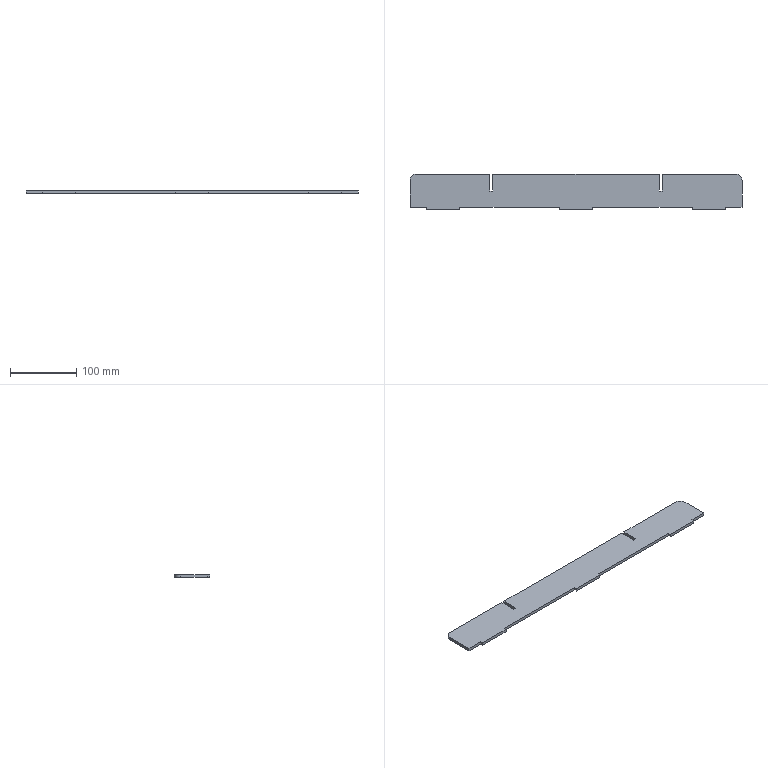Part | SolidWorks | features FlatPattern 1, SMBaseFlange 1, SheetMetal 1 | 1 solid | 28 faces | box 500 x 54 x 4.5 mm | volume 113974 mm3 | plane 26 | cylinder 2 | commonest cylinder face diameters 20 x2
STEP:
#1=CARTESIAN_POINT('',(-710.,249.731,0.));
#2=VERTEX_POINT('',#1);
#3=CARTESIAN_POINT('',(-685.,249.731,0.));
#4=VERTEX_POINT('',#3);
#5=CARTESIAN_POINT('',(-685.,249.731,0.));
#6=DIRECTION('',(1.,0.,0.));
#7=VECTOR('',#6,1000.);
#8=LINE('',#5,#7);
#9=EDGE_CURVE('',#2,#4,#8,.T.);
#10=ORIENTED_EDGE('',*,*,#9,.F.);
#11=CARTESIAN_POINT('',(-710.,249.731,-4.5));
#12=VERTEX_POINT('',#11);
#13=CARTESIAN_POINT('',(-710.,249.731,-4.5));
#14=DIRECTION('',(0.,0.,1.));
#15=VECTOR('',#14,1000.);
#16=LINE('',#13,#15);
#17=EDGE_CURVE('',#12,#2,#16,.T.);
#18=ORIENTED_EDGE('',*,*,#17,.F.);
#19=CARTESIAN_POINT('',(-685.,249.731,-4.5));
#20=VERTEX_POINT('',#19);
#21=CARTESIAN_POINT('',(-685.,249.731,-4.5));
#22=DIRECTION('',(1.,0.,0.));
#23=VECTOR('',#22,1000.);
#24=LINE('',#21,#23);
#25=EDGE_CURVE('',#12,#20,#24,.T.);
#26=ORIENTED_EDGE('',*,*,#25,.T.);
#27=CARTESIAN_POINT('',(-685.,249.731,-4.5));
#28=DIRECTION('',(0.,0.,1.));
#29=VECTOR('',#28,1000.);
#30=LINE('',#27,#29);
#31=EDGE_CURVE('',#20,#4,#30,.T.);
#32=ORIENTED_EDGE('',*,*,#31,.T.);
#33=EDGE_LOOP('',(#10,#18,#26,#32));
#34=FACE_OUTER_BOUND('',#33,.T.);
#35=CARTESIAN_POINT('',(-685.,249.731,-4.5));
#36=DIRECTION('',(0.,-1.,0.));
#37=DIRECTION('',(0.,0.,-1.));
#38=AXIS2_PLACEMENT_3D('',#35,#36,#37);
#39=PLANE('',#38);
#40=ADVANCED_FACE('',(#34),#39,.T.);
#41=CARTESIAN_POINT('',(-710.,289.731,0.));
#42=VERTEX_POINT('',#41);
#43=CARTESIAN_POINT('',(-710.,249.731,0.));
#44=DIRECTION('',(0.,-1.,0.));
#45=VECTOR('',#44,1000.);
#46=LINE('',#43,#45);
#47=EDGE_CURVE('',#42,#2,#46,.T.);
#48=ORIENTED_EDGE('',*,*,#47,.F.);
#49=CARTESIAN_POINT('',(-710.,289.731,-4.5));
#50=VERTEX_POINT('',#49);
#51=CARTESIAN_POINT('',(-710.,289.731,-4.5));
#52=DIRECTION('',(0.,0.,1.));
#53=VECTOR('',#52,1000.);
#54=LINE('',#51,#53);
#55=EDGE_CURVE('',#50,#42,#54,.T.);
#56=ORIENTED_EDGE('',*,*,#55,.F.);
#57=CARTESIAN_POINT('',(-710.,249.731,-4.5));
#58=DIRECTION('',(0.,-1.,0.));
#59=VECTOR('',#58,1000.);
#60=LINE('',#57,#59);
#61=EDGE_CURVE('',#50,#12,#60,.T.);
#62=ORIENTED_EDGE('',*,*,#61,.T.);
#63=ORIENTED_EDGE('',*,*,#17,.T.);
#64=EDGE_LOOP('',(#48,#56,#62,#63));
#65=FACE_OUTER_BOUND('',#64,.T.);
#66=CARTESIAN_POINT('',(-710.,249.731,-4.5));
#67=DIRECTION('',(-1.,0.,0.));
#68=DIRECTION('',(0.,0.,1.));
#69=AXIS2_PLACEMENT_3D('',#66,#67,#68);
#70=PLANE('',#69);
#71=ADVANCED_FACE('',(#65),#70,.T.);
#72=CARTESIAN_POINT('',(-700.,299.731,0.));
#73=VERTEX_POINT('',#72);
#74=CARTESIAN_POINT('',(-700.,289.731,0.));
#75=DIRECTION('',(0.,0.,1.));
#76=DIRECTION('',(-1.,0.,0.));
#77=AXIS2_PLACEMENT_3D('',#74,#75,#76);
#78=CIRCLE('',#77,10.);
#79=EDGE_CURVE('',#73,#42,#78,.T.);
#80=ORIENTED_EDGE('',*,*,#79,.F.);
#81=CARTESIAN_POINT('',(-700.,299.731,-4.5));
#82=VERTEX_POINT('',#81);
#83=CARTESIAN_POINT('',(-700.,299.731,-4.5));
#84=DIRECTION('',(0.,0.,1.));
#85=VECTOR('',#84,1000.);
#86=LINE('',#83,#85);
#87=EDGE_CURVE('',#82,#73,#86,.T.);
#88=ORIENTED_EDGE('',*,*,#87,.F.);
#89=CARTESIAN_POINT('',(-700.,289.731,-4.5));
#90=DIRECTION('',(0.,0.,1.));
#91=DIRECTION('',(-1.,0.,0.));
#92=AXIS2_PLACEMENT_3D('',#89,#90,#91);
#93=CIRCLE('',#92,10.);
#94=EDGE_CURVE('',#82,#50,#93,.T.);
#95=ORIENTED_EDGE('',*,*,#94,.T.);
#96=ORIENTED_EDGE('',*,*,#55,.T.);
#97=EDGE_LOOP('',(#80,#88,#95,#96));
#98=FACE_OUTER_BOUND('',#97,.T.);
#99=CARTESIAN_POINT('',(-700.,289.731,-4.5));
#100=DIRECTION('',(0.,0.,1.));
#101=DIRECTION('',(1.,0.,0.));
#102=AXIS2_PLACEMENT_3D('',#99,#100,#101);
#103=CYLINDRICAL_SURFACE('',#102,10.);
#104=ADVANCED_FACE('',(#98),#103,.T.);
#105=CARTESIAN_POINT('',(-590.,299.731,0.));
#106=VERTEX_POINT('',#105);
#107=CARTESIAN_POINT('',(-700.,299.731,0.));
#108=DIRECTION('',(-1.,0.,0.));
#109=VECTOR('',#108,1000.);
#110=LINE('',#107,#109);
#111=EDGE_CURVE('',#106,#73,#110,.T.);
#112=ORIENTED_EDGE('',*,*,#111,.F.);
#113=CARTESIAN_POINT('',(-590.,299.731,-4.5));
#114=VERTEX_POINT('',#113);
#115=CARTESIAN_POINT('',(-590.,299.731,-4.5));
#116=DIRECTION('',(0.,0.,1.));
#117=VECTOR('',#116,1000.);
#118=LINE('',#115,#117);
#119=EDGE_CURVE('',#114,#106,#118,.T.);
#120=ORIENTED_EDGE('',*,*,#119,.F.);
#121=CARTESIAN_POINT('',(-700.,299.731,-4.5));
#122=DIRECTION('',(-1.,0.,0.));
#123=VECTOR('',#122,1000.);
#124=LINE('',#121,#123);
#125=EDGE_CURVE('',#114,#82,#124,.T.);
#126=ORIENTED_EDGE('',*,*,#125,.T.);
#127=ORIENTED_EDGE('',*,*,#87,.T.);
#128=EDGE_LOOP('',(#112,#120,#126,#127));
#129=FACE_OUTER_BOUND('',#128,.T.);
#130=CARTESIAN_POINT('',(-700.,299.731,-4.5));
#131=DIRECTION('',(0.,1.,0.));
#132=DIRECTION('',(-1.,0.,0.));
#133=AXIS2_PLACEMENT_3D('',#130,#131,#132);
#134=PLANE('',#133);
#135=ADVANCED_FACE('',(#129),#134,.T.);
#136=CARTESIAN_POINT('',(-590.,274.231,0.));
#137=VERTEX_POINT('',#136);
#138=CARTESIAN_POINT('',(-590.,299.731,0.));
#139=DIRECTION('',(0.,1.,0.));
#140=VECTOR('',#139,1000.);
#141=LINE('',#138,#140);
#142=EDGE_CURVE('',#137,#106,#141,.T.);
#143=ORIENTED_EDGE('',*,*,#142,.F.);
#144=CARTESIAN_POINT('',(-590.,274.231,-4.5));
#145=VERTEX_POINT('',#144);
#146=CARTESIAN_POINT('',(-590.,274.231,-4.5));
#147=DIRECTION('',(0.,0.,1.));
#148=VECTOR('',#147,1000.);
#149=LINE('',#146,#148);
#150=EDGE_CURVE('',#145,#137,#149,.T.);
#151=ORIENTED_EDGE('',*,*,#150,.F.);
#152=CARTESIAN_POINT('',(-590.,299.731,-4.5));
#153=DIRECTION('',(0.,1.,0.));
#154=VECTOR('',#153,1000.);
#155=LINE('',#152,#154);
#156=EDGE_CURVE('',#145,#114,#155,.T.);
#157=ORIENTED_EDGE('',*,*,#156,.T.);
#158=ORIENTED_EDGE('',*,*,#119,.T.);
#159=EDGE_LOOP('',(#143,#151,#157,#158));
#160=FACE_OUTER_BOUND('',#159,.T.);
#161=CARTESIAN_POINT('',(-590.,299.731,-4.5));
#162=DIRECTION('',(1.,0.,0.));
#163=DIRECTION('',(0.,0.,-1.));
#164=AXIS2_PLACEMENT_3D('',#161,#162,#163);
#165=PLANE('',#164);
#166=ADVANCED_FACE('',(#160),#165,.T.);
#167=CARTESIAN_POINT('',(-585.5,274.231,0.));
#168=VERTEX_POINT('',#167);
#169=CARTESIAN_POINT('',(-590.,274.231,0.));
#170=DIRECTION('',(-1.,0.,0.));
#171=VECTOR('',#170,1000.);
#172=LINE('',#169,#171);
#173=EDGE_CURVE('',#168,#137,#172,.T.);
#174=ORIENTED_EDGE('',*,*,#173,.F.);
#175=CARTESIAN_POINT('',(-585.5,274.231,-4.5));
#176=VERTEX_POINT('',#175);
#177=CARTESIAN_POINT('',(-585.5,274.231,-4.5));
#178=DIRECTION('',(0.,0.,1.));
#179=VECTOR('',#178,1000.);
#180=LINE('',#177,#179);
#181=EDGE_CURVE('',#176,#168,#180,.T.);
#182=ORIENTED_EDGE('',*,*,#181,.F.);
#183=CARTESIAN_POINT('',(-590.,274.231,-4.5));
#184=DIRECTION('',(-1.,0.,0.));
#185=VECTOR('',#184,1000.);
#186=LINE('',#183,#185);
#187=EDGE_CURVE('',#176,#145,#186,.T.);
#188=ORIENTED_EDGE('',*,*,#187,.T.);
#189=ORIENTED_EDGE('',*,*,#150,.T.);
#190=EDGE_LOOP('',(#174,#182,#188,#189));
#191=FACE_OUTER_BOUND('',#190,.T.);
#192=CARTESIAN_POINT('',(-590.,274.231,-4.5));
#193=DIRECTION('',(0.,1.,0.));
#194=DIRECTION('',(0.,0.,1.));
#195=AXIS2_PLACEMENT_3D('',#192,#193,#194);
#196=PLANE('',#195);
#197=ADVANCED_FACE('',(#191),#196,.T.);
#198=CARTESIAN_POINT('',(-585.5,299.731,0.));
#199=VERTEX_POINT('',#198);
#200=CARTESIAN_POINT('',(-585.5,274.231,0.));
#201=DIRECTION('',(0.,-1.,0.));
#202=VECTOR('',#201,1000.);
#203=LINE('',#200,#202);
#204=EDGE_CURVE('',#199,#168,#203,.T.);
#205=ORIENTED_EDGE('',*,*,#204,.F.);
#206=CARTESIAN_POINT('',(-585.5,299.731,-4.5));
#207=VERTEX_POINT('',#206);
#208=CARTESIAN_POINT('',(-585.5,299.731,-4.5));
#209=DIRECTION('',(0.,0.,1.));
#210=VECTOR('',#209,1000.);
#211=LINE('',#208,#210);
#212=EDGE_CURVE('',#207,#199,#211,.T.);
#213=ORIENTED_EDGE('',*,*,#212,.F.);
#214=CARTESIAN_POINT('',(-585.5,274.231,-4.5));
#215=DIRECTION('',(0.,-1.,0.));
#216=VECTOR('',#215,1000.);
#217=LINE('',#214,#216);
#218=EDGE_CURVE('',#207,#176,#217,.T.);
#219=ORIENTED_EDGE('',*,*,#218,.T.);
#220=ORIENTED_EDGE('',*,*,#181,.T.);
#221=EDGE_LOOP('',(#205,#213,#219,#220));
#222=FACE_OUTER_BOUND('',#221,.T.);
#223=CARTESIAN_POINT('',(-585.5,274.231,-4.5));
#224=DIRECTION('',(-1.,0.,0.));
#225=DIRECTION('',(0.,0.,1.));
#226=AXIS2_PLACEMENT_3D('',#223,#224,#225);
#227=PLANE('',#226);
#228=ADVANCED_FACE('',(#222),#227,.T.);
#229=CARTESIAN_POINT('',(-334.5,299.731,0.));
#230=VERTEX_POINT('',#229);
#231=CARTESIAN_POINT('',(-585.5,299.731,0.));
#232=DIRECTION('',(-1.,0.,0.));
#233=VECTOR('',#232,1000.);
#234=LINE('',#231,#233);
#235=EDGE_CURVE('',#230,#199,#234,.T.);
#236=ORIENTED_EDGE('',*,*,#235,.F.);
#237=CARTESIAN_POINT('',(-334.5,299.731,-4.5));
#238=VERTEX_POINT('',#237);
#239=CARTESIAN_POINT('',(-334.5,299.731,-4.5));
#240=DIRECTION('',(0.,0.,1.));
#241=VECTOR('',#240,1000.);
#242=LINE('',#239,#241);
#243=EDGE_CURVE('',#238,#230,#242,.T.);
#244=ORIENTED_EDGE('',*,*,#243,.F.);
#245=CARTESIAN_POINT('',(-585.5,299.731,-4.5));
#246=DIRECTION('',(-1.,0.,0.));
#247=VECTOR('',#246,1000.);
#248=LINE('',#245,#247);
#249=EDGE_CURVE('',#238,#207,#248,.T.);
#250=ORIENTED_EDGE('',*,*,#249,.T.);
#251=ORIENTED_EDGE('',*,*,#212,.T.);
#252=EDGE_LOOP('',(#236,#244,#250,#251));
#253=FACE_OUTER_BOUND('',#252,.T.);
#254=CARTESIAN_POINT('',(-585.5,299.731,-4.5));
#255=DIRECTION('',(0.,1.,0.));
#256=DIRECTION('',(-1.,0.,0.));
#257=AXIS2_PLACEMENT_3D('',#254,#255,#256);
#258=PLANE('',#257);
#259=ADVANCED_FACE('',(#253),#258,.T.);
#260=CARTESIAN_POINT('',(-334.5,274.231,0.));
#261=VERTEX_POINT('',#260);
#262=CARTESIAN_POINT('',(-334.5,299.731,0.));
#263=DIRECTION('',(0.,1.,0.));
#264=VECTOR('',#263,1000.);
#265=LINE('',#262,#264);
#266=EDGE_CURVE('',#261,#230,#265,.T.);
#267=ORIENTED_EDGE('',*,*,#266,.F.);
#268=CARTESIAN_POINT('',(-334.5,274.231,-4.5));
#269=VERTEX_POINT('',#268);
#270=CARTESIAN_POINT('',(-334.5,274.231,-4.5));
#271=DIRECTION('',(0.,0.,1.));
#272=VECTOR('',#271,1000.);
#273=LINE('',#270,#272);
#274=EDGE_CURVE('',#269,#261,#273,.T.);
#275=ORIENTED_EDGE('',*,*,#274,.F.);
#276=CARTESIAN_POINT('',(-334.5,299.731,-4.5));
#277=DIRECTION('',(0.,1.,0.));
#278=VECTOR('',#277,1000.);
#279=LINE('',#276,#278);
#280=EDGE_CURVE('',#269,#238,#279,.T.);
#281=ORIENTED_EDGE('',*,*,#280,.T.);
#282=ORIENTED_EDGE('',*,*,#243,.T.);
#283=EDGE_LOOP('',(#267,#275,#281,#282));
#284=FACE_OUTER_BOUND('',#283,.T.);
#285=CARTESIAN_POINT('',(-334.5,299.731,-4.5));
#286=DIRECTION('',(1.,0.,0.));
#287=DIRECTION('',(0.,1.,0.));
#288=AXIS2_PLACEMENT_3D('',#285,#286,#287);
#289=PLANE('',#288);
#290=ADVANCED_FACE('',(#284),#289,.T.);
#291=CARTESIAN_POINT('',(-330.,274.231,0.));
#292=VERTEX_POINT('',#291);
#293=CARTESIAN_POINT('',(-334.5,274.231,0.));
#294=DIRECTION('',(-1.,0.,0.));
#295=VECTOR('',#294,1000.);
#296=LINE('',#293,#295);
#297=EDGE_CURVE('',#292,#261,#296,.T.);
#298=ORIENTED_EDGE('',*,*,#297,.F.);
#299=CARTESIAN_POINT('',(-330.,274.231,-4.5));
#300=VERTEX_POINT('',#299);
#301=CARTESIAN_POINT('',(-330.,274.231,-4.5));
#302=DIRECTION('',(0.,0.,1.));
#303=VECTOR('',#302,1000.);
#304=LINE('',#301,#303);
#305=EDGE_CURVE('',#300,#292,#304,.T.);
#306=ORIENTED_EDGE('',*,*,#305,.F.);
#307=CARTESIAN_POINT('',(-334.5,274.231,-4.5));
#308=DIRECTION('',(-1.,0.,0.));
#309=VECTOR('',#308,1000.);
#310=LINE('',#307,#309);
#311=EDGE_CURVE('',#300,#269,#310,.T.);
#312=ORIENTED_EDGE('',*,*,#311,.T.);
#313=ORIENTED_EDGE('',*,*,#274,.T.);
#314=EDGE_LOOP('',(#298,#306,#312,#313));
#315=FACE_OUTER_BOUND('',#314,.T.);
#316=CARTESIAN_POINT('',(-334.5,274.231,-4.5));
#317=DIRECTION('',(0.,1.,0.));
#318=DIRECTION('',(0.,0.,1.));
#319=AXIS2_PLACEMENT_3D('',#316,#317,#318);
#320=PLANE('',#319);
#321=ADVANCED_FACE('',(#315),#320,.T.);
#322=CARTESIAN_POINT('',(-330.,299.731,0.));
#323=VERTEX_POINT('',#322);
#324=CARTESIAN_POINT('',(-330.,274.231,0.));
#325=DIRECTION('',(0.,-1.,0.));
#326=VECTOR('',#325,1000.);
#327=LINE('',#324,#326);
#328=EDGE_CURVE('',#323,#292,#327,.T.);
#329=ORIENTED_EDGE('',*,*,#328,.F.);
#330=CARTESIAN_POINT('',(-330.,299.731,-4.5));
#331=VERTEX_POINT('',#330);
#332=CARTESIAN_POINT('',(-330.,299.731,-4.5));
#333=DIRECTION('',(0.,0.,1.));
#334=VECTOR('',#333,1000.);
#335=LINE('',#332,#334);
#336=EDGE_CURVE('',#331,#323,#335,.T.);
#337=ORIENTED_EDGE('',*,*,#336,.F.);
#338=CARTESIAN_POINT('',(-330.,274.231,-4.5));
#339=DIRECTION('',(0.,-1.,0.));
#340=VECTOR('',#339,1000.);
#341=LINE('',#338,#340);
#342=EDGE_CURVE('',#331,#300,#341,.T.);
#343=ORIENTED_EDGE('',*,*,#342,.T.);
#344=ORIENTED_EDGE('',*,*,#305,.T.);
#345=EDGE_LOOP('',(#329,#337,#343,#344));
#346=FACE_OUTER_BOUND('',#345,.T.);
#347=CARTESIAN_POINT('',(-330.,274.231,-4.5));
#348=DIRECTION('',(-1.,0.,0.));
#349=DIRECTION('',(0.,-1.,0.));
#350=AXIS2_PLACEMENT_3D('',#347,#348,#349);
#351=PLANE('',#350);
#352=ADVANCED_FACE('',(#346),#351,.T.);
#353=CARTESIAN_POINT('',(-220.,299.731,0.));
#354=VERTEX_POINT('',#353);
#355=CARTESIAN_POINT('',(-330.,299.731,0.));
#356=DIRECTION('',(-1.,0.,0.));
#357=VECTOR('',#356,1000.);
#358=LINE('',#355,#357);
#359=EDGE_CURVE('',#354,#323,#358,.T.);
#360=ORIENTED_EDGE('',*,*,#359,.F.);
#361=CARTESIAN_POINT('',(-220.,299.731,-4.5));
#362=VERTEX_POINT('',#361);
#363=CARTESIAN_POINT('',(-220.,299.731,-4.5));
#364=DIRECTION('',(0.,0.,1.));
#365=VECTOR('',#364,1000.);
#366=LINE('',#363,#365);
#367=EDGE_CURVE('',#362,#354,#366,.T.);
#368=ORIENTED_EDGE('',*,*,#367,.F.);
#369=CARTESIAN_POINT('',(-330.,299.731,-4.5));
#370=DIRECTION('',(-1.,0.,0.));
#371=VECTOR('',#370,1000.);
#372=LINE('',#369,#371);
#373=EDGE_CURVE('',#362,#331,#372,.T.);
#374=ORIENTED_EDGE('',*,*,#373,.T.);
#375=ORIENTED_EDGE('',*,*,#336,.T.);
#376=EDGE_LOOP('',(#360,#368,#374,#375));
#377=FACE_OUTER_BOUND('',#376,.T.);
#378=CARTESIAN_POINT('',(-330.,299.731,-4.5));
#379=DIRECTION('',(0.,1.,0.));
#380=DIRECTION('',(-1.,0.,0.));
#381=AXIS2_PLACEMENT_3D('',#378,#379,#380);
#382=PLANE('',#381);
#383=ADVANCED_FACE('',(#377),#382,.T.);
#384=CARTESIAN_POINT('',(-210.,289.731,0.));
#385=VERTEX_POINT('',#384);
#386=CARTESIAN_POINT('',(-220.,289.731,0.));
#387=DIRECTION('',(0.,0.,1.));
#388=DIRECTION('',(-1.,0.,0.));
#389=AXIS2_PLACEMENT_3D('',#386,#387,#388);
#390=CIRCLE('',#389,10.);
#391=EDGE_CURVE('',#385,#354,#390,.T.);
#392=ORIENTED_EDGE('',*,*,#391,.F.);
#393=CARTESIAN_POINT('',(-210.,289.731,-4.5));
#394=VERTEX_POINT('',#393);
#395=CARTESIAN_POINT('',(-210.,289.731,-4.5));
#396=DIRECTION('',(0.,0.,1.));
#397=VECTOR('',#396,1000.);
#398=LINE('',#395,#397);
#399=EDGE_CURVE('',#394,#385,#398,.T.);
#400=ORIENTED_EDGE('',*,*,#399,.F.);
#401=CARTESIAN_POINT('',(-220.,289.731,-4.5));
#402=DIRECTION('',(0.,0.,1.));
#403=DIRECTION('',(-1.,0.,0.));
#404=AXIS2_PLACEMENT_3D('',#401,#402,#403);
#405=CIRCLE('',#404,10.);
#406=EDGE_CURVE('',#394,#362,#405,.T.);
#407=ORIENTED_EDGE('',*,*,#406,.T.);
#408=ORIENTED_EDGE('',*,*,#367,.T.);
#409=EDGE_LOOP('',(#392,#400,#407,#408));
#410=FACE_OUTER_BOUND('',#409,.T.);
#411=CARTESIAN_POINT('',(-220.,289.731,-4.5));
#412=DIRECTION('',(0.,0.,1.));
#413=DIRECTION('',(1.,0.,0.));
#414=AXIS2_PLACEMENT_3D('',#411,#412,#413);
#415=CYLINDRICAL_SURFACE('',#414,10.);
#416=ADVANCED_FACE('',(#410),#415,.T.);
#417=CARTESIAN_POINT('',(-210.,249.731,0.));
#418=VERTEX_POINT('',#417);
#419=CARTESIAN_POINT('',(-210.,289.731,0.));
#420=DIRECTION('',(0.,1.,0.));
#421=VECTOR('',#420,1000.);
#422=LINE('',#419,#421);
#423=EDGE_CURVE('',#418,#385,#422,.T.);
#424=ORIENTED_EDGE('',*,*,#423,.F.);
#425=CARTESIAN_POINT('',(-210.,249.731,-4.5));
#426=VERTEX_POINT('',#425);
#427=CARTESIAN_POINT('',(-210.,249.731,-4.5));
#428=DIRECTION('',(0.,0.,1.));
#429=VECTOR('',#428,1000.);
#430=LINE('',#427,#429);
#431=EDGE_CURVE('',#426,#418,#430,.T.);
#432=ORIENTED_EDGE('',*,*,#431,.F.);
#433=CARTESIAN_POINT('',(-210.,289.731,-4.5));
#434=DIRECTION('',(0.,1.,0.));
#435=VECTOR('',#434,1000.);
#436=LINE('',#433,#435);
#437=EDGE_CURVE('',#426,#394,#436,.T.);
#438=ORIENTED_EDGE('',*,*,#437,.T.);
#439=ORIENTED_EDGE('',*,*,#399,.T.);
#440=EDGE_LOOP('',(#424,#432,#438,#439));
#441=FACE_OUTER_BOUND('',#440,.T.);
#442=CARTESIAN_POINT('',(-210.,289.731,-4.5));
#443=DIRECTION('',(1.,0.,0.));
#444=DIRECTION('',(0.,1.,0.));
#445=AXIS2_PLACEMENT_3D('',#442,#443,#444);
#446=PLANE('',#445);
#447=ADVANCED_FACE('',(#441),#446,.T.);
#448=CARTESIAN_POINT('',(-235.,249.731,0.));
#449=VERTEX_POINT('',#448);
#450=CARTESIAN_POINT('',(-210.,249.731,0.));
#451=DIRECTION('',(1.,0.,0.));
#452=VECTOR('',#451,1000.);
#453=LINE('',#450,#452);
#454=EDGE_CURVE('',#449,#418,#453,.T.);
#455=ORIENTED_EDGE('',*,*,#454,.F.);
#456=CARTESIAN_POINT('',(-235.,249.731,-4.5));
#457=VERTEX_POINT('',#456);
#458=CARTESIAN_POINT('',(-235.,249.731,-4.5));
#459=DIRECTION('',(0.,0.,1.));
#460=VECTOR('',#459,1000.);
#461=LINE('',#458,#460);
#462=EDGE_CURVE('',#457,#449,#461,.T.);
#463=ORIENTED_EDGE('',*,*,#462,.F.);
#464=CARTESIAN_POINT('',(-210.,249.731,-4.5));
#465=DIRECTION('',(1.,0.,0.));
#466=VECTOR('',#465,1000.);
#467=LINE('',#464,#466);
#468=EDGE_CURVE('',#457,#426,#467,.T.);
#469=ORIENTED_EDGE('',*,*,#468,.T.);
#470=ORIENTED_EDGE('',*,*,#431,.T.);
#471=EDGE_LOOP('',(#455,#463,#469,#470));
#472=FACE_OUTER_BOUND('',#471,.T.);
#473=CARTESIAN_POINT('',(-210.,249.731,-4.5));
#474=DIRECTION('',(0.,-1.,0.));
#475=DIRECTION('',(1.,0.,0.));
#476=AXIS2_PLACEMENT_3D('',#473,#474,#475);
#477=PLANE('',#476);
#478=ADVANCED_FACE('',(#472),#477,.T.);
#479=CARTESIAN_POINT('',(-235.,245.731,0.));
#480=VERTEX_POINT('',#479);
#481=CARTESIAN_POINT('',(-235.,245.731,0.));
#482=DIRECTION('',(0.,1.,0.));
#483=VECTOR('',#482,1000.);
#484=LINE('',#481,#483);
#485=EDGE_CURVE('',#480,#449,#484,.T.);
#486=ORIENTED_EDGE('',*,*,#485,.F.);
#487=CARTESIAN_POINT('',(-235.,245.731,-4.5));
#488=VERTEX_POINT('',#487);
#489=CARTESIAN_POINT('',(-235.,245.731,-4.5));
#490=DIRECTION('',(0.,0.,1.));
#491=VECTOR('',#490,1000.);
#492=LINE('',#489,#491);
#493=EDGE_CURVE('',#488,#480,#492,.T.);
#494=ORIENTED_EDGE('',*,*,#493,.F.);
#495=CARTESIAN_POINT('',(-235.,245.731,-4.5));
#496=DIRECTION('',(0.,1.,0.));
#497=VECTOR('',#496,1000.);
#498=LINE('',#495,#497);
#499=EDGE_CURVE('',#488,#457,#498,.T.);
#500=ORIENTED_EDGE('',*,*,#499,.T.);
#501=ORIENTED_EDGE('',*,*,#462,.T.);
#502=EDGE_LOOP('',(#486,#494,#500,#501));
#503=FACE_OUTER_BOUND('',#502,.T.);
#504=CARTESIAN_POINT('',(-235.,245.731,-4.5));
#505=DIRECTION('',(1.,0.,0.));
#506=DIRECTION('',(0.,0.,-1.));
#507=AXIS2_PLACEMENT_3D('',#504,#505,#506);
#508=PLANE('',#507);
#509=ADVANCED_FACE('',(#503),#508,.T.);
#510=CARTESIAN_POINT('',(-285.,245.731,0.));
#511=VERTEX_POINT('',#510);
#512=CARTESIAN_POINT('',(-285.,245.731,0.));
#513=DIRECTION('',(1.,0.,0.));
#514=VECTOR('',#513,1000.);
#515=LINE('',#512,#514);
#516=EDGE_CURVE('',#511,#480,#515,.T.);
#517=ORIENTED_EDGE('',*,*,#516,.F.);
#518=CARTESIAN_POINT('',(-285.,245.731,-4.5));
#519=VERTEX_POINT('',#518);
#520=CARTESIAN_POINT('',(-285.,245.731,-4.5));
#521=DIRECTION('',(0.,0.,1.));
#522=VECTOR('',#521,1000.);
#523=LINE('',#520,#522);
#524=EDGE_CURVE('',#519,#511,#523,.T.);
#525=ORIENTED_EDGE('',*,*,#524,.F.);
#526=CARTESIAN_POINT('',(-285.,245.731,-4.5));
#527=DIRECTION('',(1.,0.,0.));
#528=VECTOR('',#527,1000.);
#529=LINE('',#526,#528);
#530=EDGE_CURVE('',#519,#488,#529,.T.);
#531=ORIENTED_EDGE('',*,*,#530,.T.);
#532=ORIENTED_EDGE('',*,*,#493,.T.);
#533=EDGE_LOOP('',(#517,#525,#531,#532));
#534=FACE_OUTER_BOUND('',#533,.T.);
#535=CARTESIAN_POINT('',(-285.,245.731,-4.5));
#536=DIRECTION('',(0.,-1.,0.));
#537=DIRECTION('',(0.,0.,-1.));
#538=AXIS2_PLACEMENT_3D('',#535,#536,#537);
#539=PLANE('',#538);
#540=ADVANCED_FACE('',(#534),#539,.T.);
#541=CARTESIAN_POINT('',(-285.,249.731,0.));
#542=VERTEX_POINT('',#541);
#543=CARTESIAN_POINT('',(-285.,249.731,0.));
#544=DIRECTION('',(0.,-1.,0.));
#545=VECTOR('',#544,1000.);
#546=LINE('',#543,#545);
#547=EDGE_CURVE('',#542,#511,#546,.T.);
#548=ORIENTED_EDGE('',*,*,#547,.F.);
#549=CARTESIAN_POINT('',(-285.,249.731,-4.5));
#550=VERTEX_POINT('',#549);
#551=CARTESIAN_POINT('',(-285.,249.731,-4.5));
#552=DIRECTION('',(0.,0.,1.));
#553=VECTOR('',#552,1000.);
#554=LINE('',#551,#553);
#555=EDGE_CURVE('',#550,#542,#554,.T.);
#556=ORIENTED_EDGE('',*,*,#555,.F.);
#557=CARTESIAN_POINT('',(-285.,249.731,-4.5));
#558=DIRECTION('',(0.,-1.,0.));
#559=VECTOR('',#558,1000.);
#560=LINE('',#557,#559);
#561=EDGE_CURVE('',#550,#519,#560,.T.);
#562=ORIENTED_EDGE('',*,*,#561,.T.);
#563=ORIENTED_EDGE('',*,*,#524,.T.);
#564=EDGE_LOOP('',(#548,#556,#562,#563));
#565=FACE_OUTER_BOUND('',#564,.T.);
#566=CARTESIAN_POINT('',(-285.,249.731,-4.5));
#567=DIRECTION('',(-1.,0.,0.));
#568=DIRECTION('',(0.,0.,1.));
#569=AXIS2_PLACEMENT_3D('',#566,#567,#568);
#570=PLANE('',#569);
#571=ADVANCED_FACE('',(#565),#570,.T.);
#572=CARTESIAN_POINT('',(-435.,249.731,0.));
#573=VERTEX_POINT('',#572);
#574=CARTESIAN_POINT('',(-285.,249.731,0.));
#575=DIRECTION('',(1.,0.,0.));
#576=VECTOR('',#575,1000.);
#577=LINE('',#574,#576);
#578=EDGE_CURVE('',#573,#542,#577,.T.);
#579=ORIENTED_EDGE('',*,*,#578,.F.);
#580=CARTESIAN_POINT('',(-435.,249.731,-4.5));
#581=VERTEX_POINT('',#580);
#582=CARTESIAN_POINT('',(-435.,249.731,-4.5));
#583=DIRECTION('',(0.,0.,1.));
#584=VECTOR('',#583,1000.);
#585=LINE('',#582,#584);
#586=EDGE_CURVE('',#581,#573,#585,.T.);
#587=ORIENTED_EDGE('',*,*,#586,.F.);
#588=CARTESIAN_POINT('',(-285.,249.731,-4.5));
#589=DIRECTION('',(1.,0.,0.));
#590=VECTOR('',#589,1000.);
#591=LINE('',#588,#590);
#592=EDGE_CURVE('',#581,#550,#591,.T.);
#593=ORIENTED_EDGE('',*,*,#592,.T.);
#594=ORIENTED_EDGE('',*,*,#555,.T.);
#595=EDGE_LOOP('',(#579,#587,#593,#594));
#596=FACE_OUTER_BOUND('',#595,.T.);
#597=CARTESIAN_POINT('',(-285.,249.731,-4.5));
#598=DIRECTION('',(0.,-1.,0.));
#599=DIRECTION('',(1.,0.,0.));
#600=AXIS2_PLACEMENT_3D('',#597,#598,#599);
#601=PLANE('',#600);
#602=ADVANCED_FACE('',(#596),#601,.T.);
#603=CARTESIAN_POINT('',(-435.,245.731,0.));
#604=VERTEX_POINT('',#603);
#605=CARTESIAN_POINT('',(-435.,245.731,0.));
#606=DIRECTION('',(0.,1.,0.));
#607=VECTOR('',#606,1000.);
#608=LINE('',#605,#607);
#609=EDGE_CURVE('',#604,#573,#608,.T.);
#610=ORIENTED_EDGE('',*,*,#609,.F.);
#611=CARTESIAN_POINT('',(-435.,245.731,-4.5));
#612=VERTEX_POINT('',#611);
#613=CARTESIAN_POINT('',(-435.,245.731,-4.5));
#614=DIRECTION('',(0.,0.,1.));
#615=VECTOR('',#614,1000.);
#616=LINE('',#613,#615);
#617=EDGE_CURVE('',#612,#604,#616,.T.);
#618=ORIENTED_EDGE('',*,*,#617,.F.);
#619=CARTESIAN_POINT('',(-435.,245.731,-4.5));
#620=DIRECTION('',(0.,1.,0.));
#621=VECTOR('',#620,1000.);
#622=LINE('',#619,#621);
#623=EDGE_CURVE('',#612,#581,#622,.T.);
#624=ORIENTED_EDGE('',*,*,#623,.T.);
#625=ORIENTED_EDGE('',*,*,#586,.T.);
#626=EDGE_LOOP('',(#610,#618,#624,#625));
#627=FACE_OUTER_BOUND('',#626,.T.);
#628=CARTESIAN_POINT('',(-435.,245.731,-4.5));
#629=DIRECTION('',(1.,0.,0.));
#630=DIRECTION('',(0.,0.,-1.));
#631=AXIS2_PLACEMENT_3D('',#628,#629,#630);
#632=PLANE('',#631);
#633=ADVANCED_FACE('',(#627),#632,.T.);
#634=CARTESIAN_POINT('',(-485.,245.731,0.));
#635=VERTEX_POINT('',#634);
#636=CARTESIAN_POINT('',(-485.,245.731,0.));
#637=DIRECTION('',(1.,0.,0.));
#638=VECTOR('',#637,1000.);
#639=LINE('',#636,#638);
#640=EDGE_CURVE('',#635,#604,#639,.T.);
#641=ORIENTED_EDGE('',*,*,#640,.F.);
#642=CARTESIAN_POINT('',(-485.,245.731,-4.5));
#643=VERTEX_POINT('',#642);
#644=CARTESIAN_POINT('',(-485.,245.731,-4.5));
#645=DIRECTION('',(0.,0.,1.));
#646=VECTOR('',#645,1000.);
#647=LINE('',#644,#646);
#648=EDGE_CURVE('',#643,#635,#647,.T.);
#649=ORIENTED_EDGE('',*,*,#648,.F.);
#650=CARTESIAN_POINT('',(-485.,245.731,-4.5));
#651=DIRECTION('',(1.,0.,0.));
#652=VECTOR('',#651,1000.);
#653=LINE('',#650,#652);
#654=EDGE_CURVE('',#643,#612,#653,.T.);
#655=ORIENTED_EDGE('',*,*,#654,.T.);
#656=ORIENTED_EDGE('',*,*,#617,.T.);
#657=EDGE_LOOP('',(#641,#649,#655,#656));
#658=FACE_OUTER_BOUND('',#657,.T.);
#659=CARTESIAN_POINT('',(-485.,245.731,-4.5));
#660=DIRECTION('',(0.,-1.,0.));
#661=DIRECTION('',(0.,0.,-1.));
#662=AXIS2_PLACEMENT_3D('',#659,#660,#661);
#663=PLANE('',#662);
#664=ADVANCED_FACE('',(#658),#663,.T.);
#665=CARTESIAN_POINT('',(-485.,249.731,0.));
#666=VERTEX_POINT('',#665);
#667=CARTESIAN_POINT('',(-485.,249.731,0.));
#668=DIRECTION('',(0.,-1.,0.));
#669=VECTOR('',#668,1000.);
#670=LINE('',#667,#669);
#671=EDGE_CURVE('',#666,#635,#670,.T.);
#672=ORIENTED_EDGE('',*,*,#671,.F.);
#673=CARTESIAN_POINT('',(-485.,249.731,-4.5));
#674=VERTEX_POINT('',#673);
#675=CARTESIAN_POINT('',(-485.,249.731,-4.5));
#676=DIRECTION('',(0.,0.,1.));
#677=VECTOR('',#676,1000.);
#678=LINE('',#675,#677);
#679=EDGE_CURVE('',#674,#666,#678,.T.);
#680=ORIENTED_EDGE('',*,*,#679,.F.);
#681=CARTESIAN_POINT('',(-485.,249.731,-4.5));
#682=DIRECTION('',(0.,-1.,0.));
#683=VECTOR('',#682,1000.);
#684=LINE('',#681,#683);
#685=EDGE_CURVE('',#674,#643,#684,.T.);
#686=ORIENTED_EDGE('',*,*,#685,.T.);
#687=ORIENTED_EDGE('',*,*,#648,.T.);
#688=EDGE_LOOP('',(#672,#680,#686,#687));
#689=FACE_OUTER_BOUND('',#688,.T.);
#690=CARTESIAN_POINT('',(-485.,249.731,-4.5));
#691=DIRECTION('',(-1.,0.,0.));
#692=DIRECTION('',(0.,0.,1.));
#693=AXIS2_PLACEMENT_3D('',#690,#691,#692);
#694=PLANE('',#693);
#695=ADVANCED_FACE('',(#689),#694,.T.);
#696=CARTESIAN_POINT('',(-635.,249.731,0.));
#697=VERTEX_POINT('',#696);
#698=CARTESIAN_POINT('',(-485.,249.731,0.));
#699=DIRECTION('',(1.,0.,0.));
#700=VECTOR('',#699,1000.);
#701=LINE('',#698,#700);
#702=EDGE_CURVE('',#697,#666,#701,.T.);
#703=ORIENTED_EDGE('',*,*,#702,.F.);
#704=CARTESIAN_POINT('',(-635.,249.731,-4.5));
#705=VERTEX_POINT('',#704);
#706=CARTESIAN_POINT('',(-635.,249.731,-4.5));
#707=DIRECTION('',(0.,0.,1.));
#708=VECTOR('',#707,1000.);
#709=LINE('',#706,#708);
#710=EDGE_CURVE('',#705,#697,#709,.T.);
#711=ORIENTED_EDGE('',*,*,#710,.F.);
#712=CARTESIAN_POINT('',(-485.,249.731,-4.5));
#713=DIRECTION('',(1.,0.,0.));
#714=VECTOR('',#713,1000.);
#715=LINE('',#712,#714);
#716=EDGE_CURVE('',#705,#674,#715,.T.);
#717=ORIENTED_EDGE('',*,*,#716,.T.);
#718=ORIENTED_EDGE('',*,*,#679,.T.);
#719=EDGE_LOOP('',(#703,#711,#717,#718));
#720=FACE_OUTER_BOUND('',#719,.T.);
#721=CARTESIAN_POINT('',(-485.,249.731,-4.5));
#722=DIRECTION('',(0.,-1.,0.));
#723=DIRECTION('',(1.,0.,0.));
#724=AXIS2_PLACEMENT_3D('',#721,#722,#723);
#725=PLANE('',#724);
#726=ADVANCED_FACE('',(#720),#725,.T.);
#727=CARTESIAN_POINT('',(-635.,245.731,0.));
#728=VERTEX_POINT('',#727);
#729=CARTESIAN_POINT('',(-635.,245.731,0.));
#730=DIRECTION('',(0.,1.,0.));
#731=VECTOR('',#730,1000.);
#732=LINE('',#729,#731);
#733=EDGE_CURVE('',#728,#697,#732,.T.);
#734=ORIENTED_EDGE('',*,*,#733,.F.);
#735=CARTESIAN_POINT('',(-635.,245.731,-4.5));
#736=VERTEX_POINT('',#735);
#737=CARTESIAN_POINT('',(-635.,245.731,-4.5));
#738=DIRECTION('',(0.,0.,1.));
#739=VECTOR('',#738,1000.);
#740=LINE('',#737,#739);
#741=EDGE_CURVE('',#736,#728,#740,.T.);
#742=ORIENTED_EDGE('',*,*,#741,.F.);
#743=CARTESIAN_POINT('',(-635.,245.731,-4.5));
#744=DIRECTION('',(0.,1.,0.));
#745=VECTOR('',#744,1000.);
#746=LINE('',#743,#745);
#747=EDGE_CURVE('',#736,#705,#746,.T.);
#748=ORIENTED_EDGE('',*,*,#747,.T.);
#749=ORIENTED_EDGE('',*,*,#710,.T.);
#750=EDGE_LOOP('',(#734,#742,#748,#749));
#751=FACE_OUTER_BOUND('',#750,.T.);
#752=CARTESIAN_POINT('',(-635.,245.731,-4.5));
#753=DIRECTION('',(1.,0.,0.));
#754=DIRECTION('',(0.,0.,-1.));
#755=AXIS2_PLACEMENT_3D('',#752,#753,#754);
#756=PLANE('',#755);
#757=ADVANCED_FACE('',(#751),#756,.T.);
#758=CARTESIAN_POINT('',(-685.,245.731,0.));
#759=VERTEX_POINT('',#758);
#760=CARTESIAN_POINT('',(-685.,245.731,0.));
#761=DIRECTION('',(1.,0.,0.));
#762=VECTOR('',#761,1000.);
#763=LINE('',#760,#762);
#764=EDGE_CURVE('',#759,#728,#763,.T.);
#765=ORIENTED_EDGE('',*,*,#764,.F.);
#766=CARTESIAN_POINT('',(-685.,245.731,-4.5));
#767=VERTEX_POINT('',#766);
#768=CARTESIAN_POINT('',(-685.,245.731,-4.5));
#769=DIRECTION('',(0.,0.,1.));
#770=VECTOR('',#769,1000.);
#771=LINE('',#768,#770);
#772=EDGE_CURVE('',#767,#759,#771,.T.);
#773=ORIENTED_EDGE('',*,*,#772,.F.);
#774=CARTESIAN_POINT('',(-685.,245.731,-4.5));
#775=DIRECTION('',(1.,0.,0.));
#776=VECTOR('',#775,1000.);
#777=LINE('',#774,#776);
#778=EDGE_CURVE('',#767,#736,#777,.T.);
#779=ORIENTED_EDGE('',*,*,#778,.T.);
#780=ORIENTED_EDGE('',*,*,#741,.T.);
#781=EDGE_LOOP('',(#765,#773,#779,#780));
#782=FACE_OUTER_BOUND('',#781,.T.);
#783=CARTESIAN_POINT('',(-685.,245.731,-4.5));
#784=DIRECTION('',(0.,-1.,0.));
#785=DIRECTION('',(0.,0.,-1.));
#786=AXIS2_PLACEMENT_3D('',#783,#784,#785);
#787=PLANE('',#786);
#788=ADVANCED_FACE('',(#782),#787,.T.);
#789=CARTESIAN_POINT('',(-685.,249.731,0.));
#790=DIRECTION('',(0.,-1.,0.));
#791=VECTOR('',#790,1000.);
#792=LINE('',#789,#791);
#793=EDGE_CURVE('',#4,#759,#792,.T.);
#794=ORIENTED_EDGE('',*,*,#793,.F.);
#795=ORIENTED_EDGE('',*,*,#31,.F.);
#796=CARTESIAN_POINT('',(-685.,249.731,-4.5));
#797=DIRECTION('',(0.,-1.,0.));
#798=VECTOR('',#797,1000.);
#799=LINE('',#796,#798);
#800=EDGE_CURVE('',#20,#767,#799,.T.);
#801=ORIENTED_EDGE('',*,*,#800,.T.);
#802=ORIENTED_EDGE('',*,*,#772,.T.);
#803=EDGE_LOOP('',(#794,#795,#801,#802));
#804=FACE_OUTER_BOUND('',#803,.T.);
#805=CARTESIAN_POINT('',(-685.,249.731,-4.5));
#806=DIRECTION('',(-1.,0.,0.));
#807=DIRECTION('',(0.,0.,1.));
#808=AXIS2_PLACEMENT_3D('',#805,#806,#807);
#809=PLANE('',#808);
#810=ADVANCED_FACE('',(#804),#809,.T.);
#811=ORIENTED_EDGE('',*,*,#25,.F.);
#812=ORIENTED_EDGE('',*,*,#61,.F.);
#813=ORIENTED_EDGE('',*,*,#94,.F.);
#814=ORIENTED_EDGE('',*,*,#125,.F.);
#815=ORIENTED_EDGE('',*,*,#156,.F.);
#816=ORIENTED_EDGE('',*,*,#187,.F.);
#817=ORIENTED_EDGE('',*,*,#218,.F.);
#818=ORIENTED_EDGE('',*,*,#249,.F.);
#819=ORIENTED_EDGE('',*,*,#280,.F.);
#820=ORIENTED_EDGE('',*,*,#311,.F.);
#821=ORIENTED_EDGE('',*,*,#342,.F.);
#822=ORIENTED_EDGE('',*,*,#373,.F.);
#823=ORIENTED_EDGE('',*,*,#406,.F.);
#824=ORIENTED_EDGE('',*,*,#437,.F.);
#825=ORIENTED_EDGE('',*,*,#468,.F.);
#826=ORIENTED_EDGE('',*,*,#499,.F.);
#827=ORIENTED_EDGE('',*,*,#530,.F.);
#828=ORIENTED_EDGE('',*,*,#561,.F.);
#829=ORIENTED_EDGE('',*,*,#592,.F.);
#830=ORIENTED_EDGE('',*,*,#623,.F.);
#831=ORIENTED_EDGE('',*,*,#654,.F.);
#832=ORIENTED_EDGE('',*,*,#685,.F.);
#833=ORIENTED_EDGE('',*,*,#716,.F.);
#834=ORIENTED_EDGE('',*,*,#747,.F.);
#835=ORIENTED_EDGE('',*,*,#778,.F.);
#836=ORIENTED_EDGE('',*,*,#800,.F.);
#837=EDGE_LOOP('',(#811,#812,#813,#814,#815,#816,#817,#818,#819,#820,#821,#822,#823,#824,#825,#826,#827,#828,#829,#830,#831,#832,#833,#834,#835,#836));
#838=FACE_OUTER_BOUND('',#837,.T.);
#839=CARTESIAN_POINT('',(-700.,289.731,-4.5));
#840=DIRECTION('',(0.,0.,-1.));
#841=DIRECTION('',(-1.,0.,0.));
#842=AXIS2_PLACEMENT_3D('',#839,#840,#841);
#843=PLANE('',#842);
#844=ADVANCED_FACE('',(#838),#843,.T.);
#845=ORIENTED_EDGE('',*,*,#9,.T.);
#846=ORIENTED_EDGE('',*,*,#793,.T.);
#847=ORIENTED_EDGE('',*,*,#764,.T.);
#848=ORIENTED_EDGE('',*,*,#733,.T.);
#849=ORIENTED_EDGE('',*,*,#702,.T.);
#850=ORIENTED_EDGE('',*,*,#671,.T.);
#851=ORIENTED_EDGE('',*,*,#640,.T.);
#852=ORIENTED_EDGE('',*,*,#609,.T.);
#853=ORIENTED_EDGE('',*,*,#578,.T.);
#854=ORIENTED_EDGE('',*,*,#547,.T.);
#855=ORIENTED_EDGE('',*,*,#516,.T.);
#856=ORIENTED_EDGE('',*,*,#485,.T.);
#857=ORIENTED_EDGE('',*,*,#454,.T.);
#858=ORIENTED_EDGE('',*,*,#423,.T.);
#859=ORIENTED_EDGE('',*,*,#391,.T.);
#860=ORIENTED_EDGE('',*,*,#359,.T.);
#861=ORIENTED_EDGE('',*,*,#328,.T.);
#862=ORIENTED_EDGE('',*,*,#297,.T.);
#863=ORIENTED_EDGE('',*,*,#266,.T.);
#864=ORIENTED_EDGE('',*,*,#235,.T.);
#865=ORIENTED_EDGE('',*,*,#204,.T.);
#866=ORIENTED_EDGE('',*,*,#173,.T.);
#867=ORIENTED_EDGE('',*,*,#142,.T.);
#868=ORIENTED_EDGE('',*,*,#111,.T.);
#869=ORIENTED_EDGE('',*,*,#79,.T.);
#870=ORIENTED_EDGE('',*,*,#47,.T.);
#871=EDGE_LOOP('',(#845,#846,#847,#848,#849,#850,#851,#852,#853,#854,#855,#856,#857,#858,#859,#860,#861,#862,#863,#864,#865,#866,#867,#868,#869,#870));
#872=FACE_OUTER_BOUND('',#871,.T.);
#873=CARTESIAN_POINT('',(-700.,289.731,0.));
#874=DIRECTION('',(0.,0.,-1.));
#875=DIRECTION('',(-1.,0.,0.));
#876=AXIS2_PLACEMENT_3D('',#873,#874,#875);
#877=PLANE('',#876);
#878=ADVANCED_FACE('',(#872),#877,.F.);
#879=CLOSED_SHELL('',(#40,#71,#104,#135,#166,#197,#228,#259,#290,#321,#352,#383,#416,#447,#478,#509,#540,#571,#602,#633,#664,#695,#726,#757,#788,#810,#844,#878));
#880=MANIFOLD_SOLID_BREP('',#879);
#881=CARTESIAN_POINT('',(0.,0.,0.));
#882=DIRECTION('',(0.,0.,1.));
#883=DIRECTION('',(1.,0.,0.));
#884=AXIS2_PLACEMENT_3D('',#881,#882,#883);
#885=(LENGTH_UNIT()NAMED_UNIT(*)SI_UNIT(.MILLI.,.METRE.));
#886=UNCERTAINTY_MEASURE_WITH_UNIT(LENGTH_MEASURE(0.00001),#885,'','');
#887=(NAMED_UNIT(*)PLANE_ANGLE_UNIT()SI_UNIT($,.RADIAN.));
#888=(NAMED_UNIT(*)SI_UNIT($,.STERADIAN.)SOLID_ANGLE_UNIT());
#889=(GEOMETRIC_REPRESENTATION_CONTEXT(3)GLOBAL_UNCERTAINTY_ASSIGNED_CONTEXT((#886))GLOBAL_UNIT_ASSIGNED_CONTEXT((#885,#887,#888))REPRESENTATION_CONTEXT('',''));
#890=ADVANCED_BREP_SHAPE_REPRESENTATION('',(#880,#884),#889);